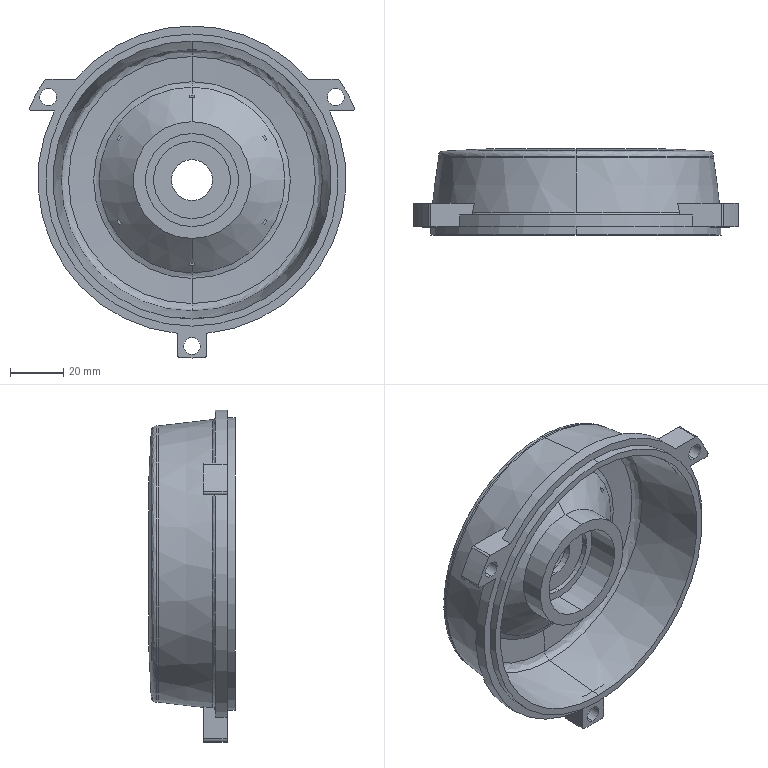Part | SolidWorks | features BaseBody 1 | 1 solid | 145 faces | box 122.449 x 32.5 x 125 mm | volume 76079 mm3 | plane 64 | cylinder 48 | spline 17 | cone 16 | commonest cylinder face diameters 64 x9 2 x6 6.3 x6 104 x6 134 x4 116 x3